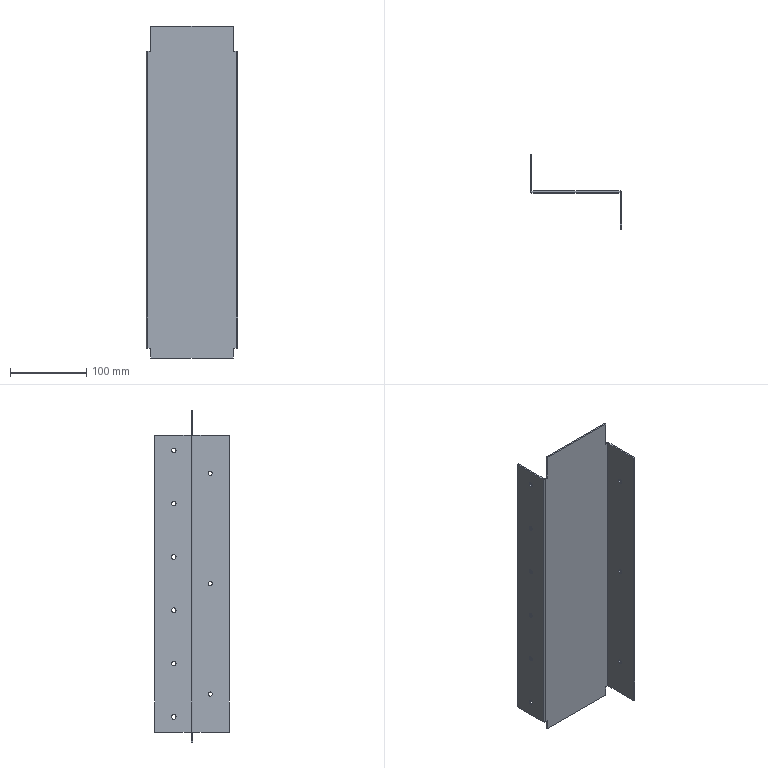Part | STEP file | SX-003-03 | 1 solid | 48 faces | box 120 x 98 x 436 mm | volume 177136 mm3 | plane 26 | cylinder 22 | commonest cylinder face diameters 6 x12 5.4 x6 0.4 x2 4.4 x2